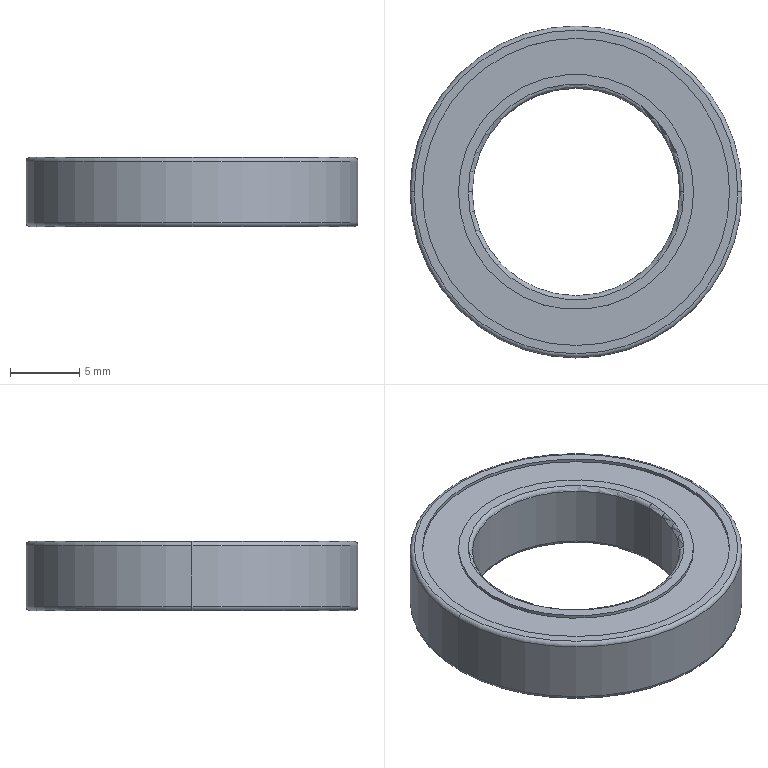Part | STEP file | B6802ZZ_C-B6802ZZ | 1 solid | 26 faces | box 24 x 24 x 5 mm | volume 1300 mm3 | cylinder 12 | torus 8 | plane 6 | commonest cylinder face diameters 17 x4 22.2 x4 15 x2 24 x2